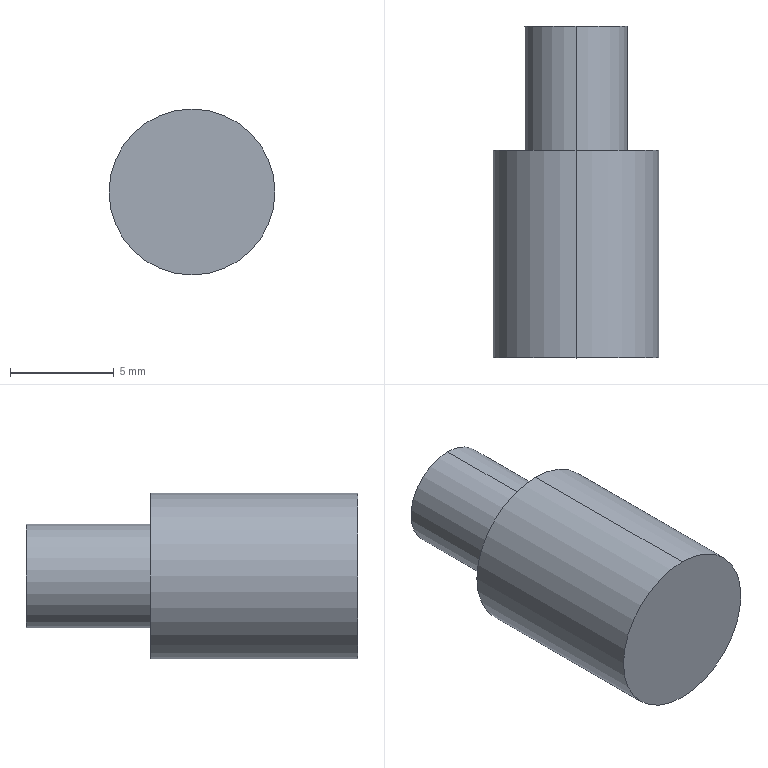Part | SolidWorks | features BaseBody 1 | 1 solid | 7 faces | box 8 x 16 x 8 mm | volume 620.465 mm3 | cylinder 4 | plane 3 | commonest cylinder face diameters 5 x2 8 x2
STEP:
#1=CARTESIAN_POINT('',(0.,-5.,4.));
#2=VERTEX_POINT('',#1);
#3=CARTESIAN_POINT('',(0.,-5.,-4.));
#4=VERTEX_POINT('',#3);
#5=CARTESIAN_POINT('',(0.,-5.,0.));
#6=DIRECTION('',(0.,1.,0.));
#7=DIRECTION('',(0.,0.,1.));
#8=AXIS2_PLACEMENT_3D('',#5,#6,#7);
#9=CIRCLE('',#8,4.);
#10=EDGE_CURVE('',#2,#4,#9,.T.);
#11=ORIENTED_EDGE('',*,*,#10,.T.);
#12=CARTESIAN_POINT('',(0.,5.,-4.));
#13=VERTEX_POINT('',#12);
#14=CARTESIAN_POINT('',(0.,-5.,-4.));
#15=DIRECTION('',(0.,1.,0.));
#16=VECTOR('',#15,1000.);
#17=LINE('',#14,#16);
#18=EDGE_CURVE('',#4,#13,#17,.T.);
#19=ORIENTED_EDGE('',*,*,#18,.T.);
#20=CARTESIAN_POINT('',(0.,5.,4.));
#21=VERTEX_POINT('',#20);
#22=CARTESIAN_POINT('',(0.,5.,0.));
#23=DIRECTION('',(0.,-1.,0.));
#24=DIRECTION('',(0.,0.,1.));
#25=AXIS2_PLACEMENT_3D('',#22,#23,#24);
#26=CIRCLE('',#25,4.);
#27=EDGE_CURVE('',#13,#21,#26,.T.);
#28=ORIENTED_EDGE('',*,*,#27,.T.);
#29=CARTESIAN_POINT('',(0.,-5.,4.));
#30=DIRECTION('',(0.,1.,0.));
#31=VECTOR('',#30,1000.);
#32=LINE('',#29,#31);
#33=EDGE_CURVE('',#2,#21,#32,.T.);
#34=ORIENTED_EDGE('',*,*,#33,.F.);
#35=EDGE_LOOP('',(#11,#19,#28,#34));
#36=FACE_OUTER_BOUND('',#35,.T.);
#37=CARTESIAN_POINT('',(0.,-5.,0.));
#38=DIRECTION('',(0.,1.,0.));
#39=DIRECTION('',(0.,0.,1.));
#40=AXIS2_PLACEMENT_3D('',#37,#38,#39);
#41=CYLINDRICAL_SURFACE('',#40,4.);
#42=ADVANCED_FACE('',(#36),#41,.T.);
#43=CARTESIAN_POINT('',(0.,5.,-2.5));
#44=VERTEX_POINT('',#43);
#45=CARTESIAN_POINT('',(0.,5.,2.5));
#46=VERTEX_POINT('',#45);
#47=CARTESIAN_POINT('',(0.,5.,0.));
#48=DIRECTION('',(0.,-1.,0.));
#49=DIRECTION('',(0.,0.,1.));
#50=AXIS2_PLACEMENT_3D('',#47,#48,#49);
#51=CIRCLE('',#50,2.5);
#52=EDGE_CURVE('',#44,#46,#51,.T.);
#53=ORIENTED_EDGE('',*,*,#52,.F.);
#54=CARTESIAN_POINT('',(0.,11.,-2.5));
#55=VERTEX_POINT('',#54);
#56=CARTESIAN_POINT('',(0.,5.,-2.5));
#57=DIRECTION('',(0.,1.,0.));
#58=VECTOR('',#57,1000.);
#59=LINE('',#56,#58);
#60=EDGE_CURVE('',#44,#55,#59,.T.);
#61=ORIENTED_EDGE('',*,*,#60,.T.);
#62=CARTESIAN_POINT('',(0.,11.,2.5));
#63=VERTEX_POINT('',#62);
#64=CARTESIAN_POINT('',(0.,11.,0.));
#65=DIRECTION('',(0.,-1.,0.));
#66=DIRECTION('',(0.,0.,1.));
#67=AXIS2_PLACEMENT_3D('',#64,#65,#66);
#68=CIRCLE('',#67,2.5);
#69=EDGE_CURVE('',#55,#63,#68,.T.);
#70=ORIENTED_EDGE('',*,*,#69,.T.);
#71=CARTESIAN_POINT('',(0.,5.,2.5));
#72=DIRECTION('',(0.,1.,0.));
#73=VECTOR('',#72,1000.);
#74=LINE('',#71,#73);
#75=EDGE_CURVE('',#46,#63,#74,.T.);
#76=ORIENTED_EDGE('',*,*,#75,.F.);
#77=EDGE_LOOP('',(#53,#61,#70,#76));
#78=FACE_OUTER_BOUND('',#77,.T.);
#79=CARTESIAN_POINT('',(0.,5.,0.));
#80=DIRECTION('',(0.,1.,0.));
#81=DIRECTION('',(0.,0.,1.));
#82=AXIS2_PLACEMENT_3D('',#79,#80,#81);
#83=CYLINDRICAL_SURFACE('',#82,2.5);
#84=ADVANCED_FACE('',(#78),#83,.T.);
#85=ORIENTED_EDGE('',*,*,#18,.F.);
#86=CARTESIAN_POINT('',(0.,-5.,0.));
#87=DIRECTION('',(0.,1.,0.));
#88=DIRECTION('',(0.,0.,1.));
#89=AXIS2_PLACEMENT_3D('',#86,#87,#88);
#90=CIRCLE('',#89,4.);
#91=EDGE_CURVE('',#4,#2,#90,.T.);
#92=ORIENTED_EDGE('',*,*,#91,.T.);
#93=ORIENTED_EDGE('',*,*,#33,.T.);
#94=CARTESIAN_POINT('',(0.,5.,0.));
#95=DIRECTION('',(0.,-1.,0.));
#96=DIRECTION('',(0.,0.,1.));
#97=AXIS2_PLACEMENT_3D('',#94,#95,#96);
#98=CIRCLE('',#97,4.);
#99=EDGE_CURVE('',#21,#13,#98,.T.);
#100=ORIENTED_EDGE('',*,*,#99,.T.);
#101=EDGE_LOOP('',(#85,#92,#93,#100));
#102=FACE_OUTER_BOUND('',#101,.T.);
#103=CARTESIAN_POINT('',(0.,-5.,0.));
#104=DIRECTION('',(0.,1.,0.));
#105=DIRECTION('',(0.,0.,1.));
#106=AXIS2_PLACEMENT_3D('',#103,#104,#105);
#107=CYLINDRICAL_SURFACE('',#106,4.);
#108=ADVANCED_FACE('',(#102),#107,.T.);
#109=ORIENTED_EDGE('',*,*,#10,.F.);
#110=ORIENTED_EDGE('',*,*,#91,.F.);
#111=EDGE_LOOP('',(#109,#110));
#112=FACE_OUTER_BOUND('',#111,.T.);
#113=CARTESIAN_POINT('',(0.,-5.,0.));
#114=DIRECTION('',(0.,1.,0.));
#115=DIRECTION('',(0.,0.,1.));
#116=AXIS2_PLACEMENT_3D('',#113,#114,#115);
#117=PLANE('',#116);
#118=ADVANCED_FACE('',(#112),#117,.F.);
#119=CARTESIAN_POINT('',(0.,5.,0.));
#120=DIRECTION('',(0.,-1.,0.));
#121=DIRECTION('',(0.,0.,1.));
#122=AXIS2_PLACEMENT_3D('',#119,#120,#121);
#123=CIRCLE('',#122,2.5);
#124=EDGE_CURVE('',#46,#44,#123,.T.);
#125=ORIENTED_EDGE('',*,*,#124,.T.);
#126=ORIENTED_EDGE('',*,*,#52,.T.);
#127=EDGE_LOOP('',(#125,#126));
#128=FACE_BOUND('',#127,.T.);
#129=ORIENTED_EDGE('',*,*,#99,.F.);
#130=ORIENTED_EDGE('',*,*,#27,.F.);
#131=EDGE_LOOP('',(#129,#130));
#132=FACE_OUTER_BOUND('',#131,.T.);
#133=CARTESIAN_POINT('',(0.,5.,0.));
#134=DIRECTION('',(0.,1.,0.));
#135=DIRECTION('',(0.,0.,1.));
#136=AXIS2_PLACEMENT_3D('',#133,#134,#135);
#137=PLANE('',#136);
#138=ADVANCED_FACE('',(#128,#132),#137,.T.);
#139=ORIENTED_EDGE('',*,*,#60,.F.);
#140=ORIENTED_EDGE('',*,*,#124,.F.);
#141=ORIENTED_EDGE('',*,*,#75,.T.);
#142=CARTESIAN_POINT('',(0.,11.,0.));
#143=DIRECTION('',(0.,-1.,0.));
#144=DIRECTION('',(0.,0.,1.));
#145=AXIS2_PLACEMENT_3D('',#142,#143,#144);
#146=CIRCLE('',#145,2.5);
#147=EDGE_CURVE('',#63,#55,#146,.T.);
#148=ORIENTED_EDGE('',*,*,#147,.T.);
#149=EDGE_LOOP('',(#139,#140,#141,#148));
#150=FACE_OUTER_BOUND('',#149,.T.);
#151=CARTESIAN_POINT('',(0.,5.,0.));
#152=DIRECTION('',(0.,1.,0.));
#153=DIRECTION('',(0.,0.,1.));
#154=AXIS2_PLACEMENT_3D('',#151,#152,#153);
#155=CYLINDRICAL_SURFACE('',#154,2.5);
#156=ADVANCED_FACE('',(#150),#155,.T.);
#157=ORIENTED_EDGE('',*,*,#147,.F.);
#158=ORIENTED_EDGE('',*,*,#69,.F.);
#159=EDGE_LOOP('',(#157,#158));
#160=FACE_OUTER_BOUND('',#159,.T.);
#161=CARTESIAN_POINT('',(0.,11.,0.));
#162=DIRECTION('',(0.,1.,0.));
#163=DIRECTION('',(0.,0.,1.));
#164=AXIS2_PLACEMENT_3D('',#161,#162,#163);
#165=PLANE('',#164);
#166=ADVANCED_FACE('',(#160),#165,.T.);
#167=CLOSED_SHELL('',(#42,#84,#108,#118,#138,#156,#166));
#168=MANIFOLD_SOLID_BREP('',#167);
#169=CARTESIAN_POINT('',(0.,0.,0.));
#170=DIRECTION('',(0.,0.,1.));
#171=DIRECTION('',(1.,0.,0.));
#172=AXIS2_PLACEMENT_3D('',#169,#170,#171);
#173=(LENGTH_UNIT()NAMED_UNIT(*)SI_UNIT(.MILLI.,.METRE.));
#174=UNCERTAINTY_MEASURE_WITH_UNIT(LENGTH_MEASURE(0.00001),#173,'','');
#175=(NAMED_UNIT(*)PLANE_ANGLE_UNIT()SI_UNIT($,.RADIAN.));
#176=(NAMED_UNIT(*)SI_UNIT($,.STERADIAN.)SOLID_ANGLE_UNIT());
#177=(GEOMETRIC_REPRESENTATION_CONTEXT(3)GLOBAL_UNCERTAINTY_ASSIGNED_CONTEXT((#174))GLOBAL_UNIT_ASSIGNED_CONTEXT((#173,#175,#176))REPRESENTATION_CONTEXT('',''));
#178=ADVANCED_BREP_SHAPE_REPRESENTATION('',(#168,#172),#177);